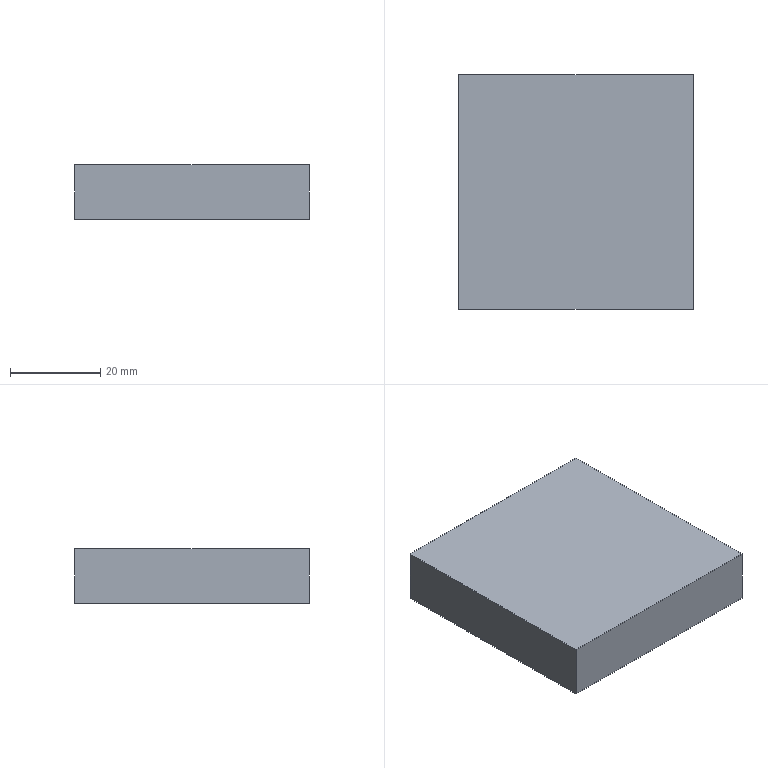NC program | NX | posted with a generic post | part box 52 x 52 x 12 mm
Lines 2514 to 2608 of 2608:
(PLANAR_MILL_1_COPY , TOOL : 倒角D3-90度)
N5008 T05 M6
N5010 G53
N5012 G17 G0 G90 X-16.921 Y12.998 S3000 M3
N5014 G43 Z30. H5
N5016 Z1.
N5018 G94 G1 Z-1. F800.
N5020 G3 X-14.938 Y10.981 R2.
N5022 G1 X-12.905 Y10.963
N5024 G3 X-10.736 Y13.094 R2.15
N5026 G1 X-10.701 Y17.161
N5028 G2 X-9.28 Y19.394 R2.5
N5030 X9.617 Y19.229 R21.5
N5032 X10.999 Y16.972 R2.5
N5034 G1 X10.963 Y12.905
N5036 G3 X13.094 Y10.736 R2.15
N5038 G1 X17.161 Y10.701
N5040 G2 X19.394 Y9.28 R2.5
N5042 X19.229 Y-9.617 R21.5
N5044 X16.972 Y-10.999 R2.5
N5046 G1 X12.905 Y-10.963
N5048 G3 X10.736 Y-13.094 R2.15
N5050 G1 X10.701 Y-17.161
N5052 G2 X9.28 Y-19.394 R2.5
N5054 X-9.617 Y-19.229 R21.5
N5056 X-10.999 Y-16.972 R2.5
N5058 G1 X-10.963 Y-12.905
N5060 G3 X-13.094 Y-10.736 R2.15
N5062 G1 X-17.161 Y-10.701
N5064 G2 X-19.394 Y-9.28 R2.5
N5066 X-19.229 Y9.617 R21.5
N5068 X-16.972 Y10.999 R2.5
N5070 G1 X-14.938 Y10.981
N5072 G3 X-12.921 Y12.963 R2.
N5074 G1 Z1.
N5076 G0 Z30.
(PLANAR_MILL_1_COPY_COPY , TOOL : 倒角D3-90度)
N5078 X-10.562 Y2.
N5080 Z1.
N5082 G1 Z-1.
N5084 X-10.75
N5086 G3 X-12.75 Y0. R2.
N5088 X0. Y-12.75 R12.75
N5090 X-12.75 Y0. R-12.75
N5092 X-10.75 Y-2. R2.
N5094 G1 X-10.562
N5096 Z1.
N5098 G0 Z30.
N5100 M5
(DRILLING , TOOL : 倒角D10-90度)
N5102 T03 M6
N5104 G53
N5106 G17 G0 G90 X-17.5 Y0. S1600 M3
N5108 G43 Z3. H3
N5110 G94 G81 G99 Z-4.15 F200. R3.
N5112 X0. Y17.5
N5114 X17.5 Y0.
N5116 X0. Y-17.5
N5118 G80
N5120 M5
(DRILLING_COPY , TOOL : 钻头D3.3-45-73)
N5122 T04 M6
N5124 G53
N5126 G17 G0 G90 X-17.5 Y0. S1600 M3
N5128 G43 Z3. H4
N5130 G94 G81 G99 Z-6. F250. R3.
N5132 X0. Y17.5
N5134 X17.5 Y0.
N5136 X0. Y-17.5
N5138 G80
N5140 M5
(PLANAR_MILL_COPY , TOOL : D50面刀)
N5142 T01 M6
N5144 G53
N5146 G17 G0 G90 X54.5 Y2.5 S4500 M3
N5148 G43 Z30. H1
N5150 Z3.
N5152 G94 G1 Z0. F800.
N5154 X27.5
N5156 X-27.5
N5158 X-54.5
N5160 Z3.
N5162 G0 Z30.
N5164 M5
N5166 M2